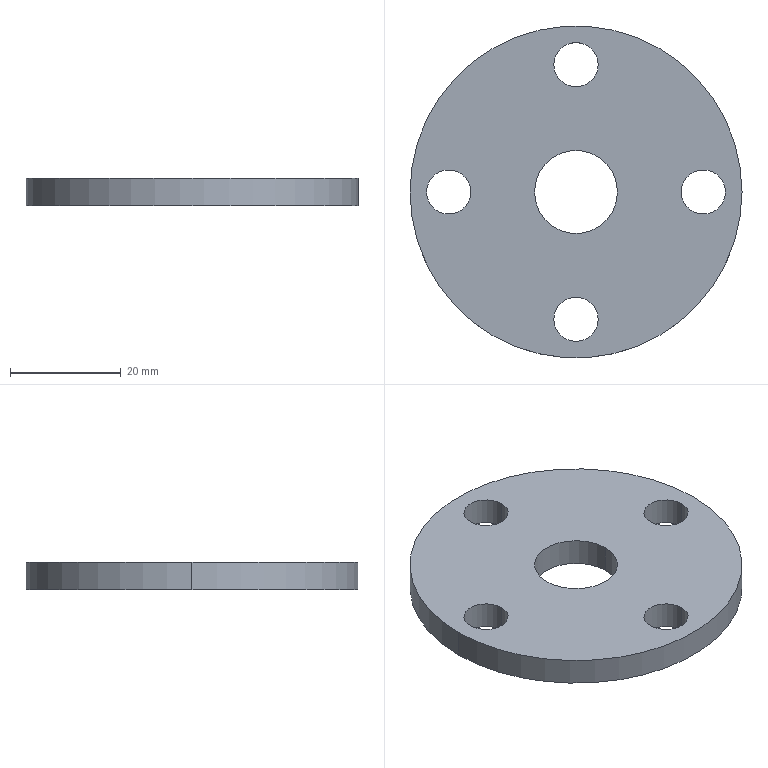Part | NX | features BREP 1 | 1 solid | 14 faces | box 60 x 60 x 5 mm | volume 12248 mm3 | cylinder 12 | plane 2 | commonest cylinder face diameters 8 x8 15 x2 60 x2
STEP:
#1=CARTESIAN_POINT('',(-27.,0.,5.));
#2=VERTEX_POINT('',#1);
#3=CARTESIAN_POINT('',(-19.,0.,5.));
#4=VERTEX_POINT('',#3);
#5=CARTESIAN_POINT('',(-23.,0.,5.));
#6=DIRECTION('',(0.,0.,1.));
#7=DIRECTION('',(1.,0.,0.));
#8=AXIS2_PLACEMENT_3D('',#5,#6,#7);
#9=CIRCLE('',#8,4.);
#10=EDGE_CURVE('',#2,#4,#9,.T.);
#11=ORIENTED_EDGE('',*,*,#10,.T.);
#12=CARTESIAN_POINT('',(-19.,0.,0.));
#13=VERTEX_POINT('',#12);
#14=CARTESIAN_POINT('',(-19.,0.,5.));
#15=DIRECTION('',(0.,0.,-1.));
#16=VECTOR('',#15,1000.);
#17=LINE('',#14,#16);
#18=EDGE_CURVE('',#13,#4,#17,.F.);
#19=ORIENTED_EDGE('',*,*,#18,.F.);
#20=CARTESIAN_POINT('',(-27.,0.,0.));
#21=VERTEX_POINT('',#20);
#22=CARTESIAN_POINT('',(-23.,0.,0.));
#23=DIRECTION('',(0.,0.,1.));
#24=DIRECTION('',(1.,0.,0.));
#25=AXIS2_PLACEMENT_3D('',#22,#23,#24);
#26=CIRCLE('',#25,4.);
#27=EDGE_CURVE('',#21,#13,#26,.T.);
#28=ORIENTED_EDGE('',*,*,#27,.F.);
#29=CARTESIAN_POINT('',(-27.,0.,5.));
#30=DIRECTION('',(0.,0.,-1.));
#31=VECTOR('',#30,1000.);
#32=LINE('',#29,#31);
#33=EDGE_CURVE('',#21,#2,#32,.F.);
#34=ORIENTED_EDGE('',*,*,#33,.T.);
#35=EDGE_LOOP('',(#11,#19,#28,#34));
#36=FACE_BOUND('',#35,.T.);
#37=CARTESIAN_POINT('',(-23.,0.,5.));
#38=DIRECTION('',(0.,0.,-1.));
#39=DIRECTION('',(1.,0.,0.));
#40=AXIS2_PLACEMENT_3D('',#37,#38,#39);
#41=CYLINDRICAL_SURFACE('',#40,4.);
#42=ADVANCED_FACE('',(#36),#41,.F.);
#43=CARTESIAN_POINT('',(-4.,-23.,5.));
#44=VERTEX_POINT('',#43);
#45=CARTESIAN_POINT('',(4.,-23.,5.));
#46=VERTEX_POINT('',#45);
#47=CARTESIAN_POINT('',(0.,-23.,5.));
#48=DIRECTION('',(0.,0.,1.));
#49=DIRECTION('',(1.,0.,0.));
#50=AXIS2_PLACEMENT_3D('',#47,#48,#49);
#51=CIRCLE('',#50,4.);
#52=EDGE_CURVE('',#44,#46,#51,.T.);
#53=ORIENTED_EDGE('',*,*,#52,.T.);
#54=CARTESIAN_POINT('',(4.,-23.,0.));
#55=VERTEX_POINT('',#54);
#56=CARTESIAN_POINT('',(4.,-23.,5.));
#57=DIRECTION('',(0.,0.,-1.));
#58=VECTOR('',#57,1000.);
#59=LINE('',#56,#58);
#60=EDGE_CURVE('',#55,#46,#59,.F.);
#61=ORIENTED_EDGE('',*,*,#60,.F.);
#62=CARTESIAN_POINT('',(-4.,-23.,0.));
#63=VERTEX_POINT('',#62);
#64=CARTESIAN_POINT('',(0.,-23.,0.));
#65=DIRECTION('',(0.,0.,1.));
#66=DIRECTION('',(1.,0.,0.));
#67=AXIS2_PLACEMENT_3D('',#64,#65,#66);
#68=CIRCLE('',#67,4.);
#69=EDGE_CURVE('',#63,#55,#68,.T.);
#70=ORIENTED_EDGE('',*,*,#69,.F.);
#71=CARTESIAN_POINT('',(-4.,-23.,5.));
#72=DIRECTION('',(0.,0.,-1.));
#73=VECTOR('',#72,1000.);
#74=LINE('',#71,#73);
#75=EDGE_CURVE('',#63,#44,#74,.F.);
#76=ORIENTED_EDGE('',*,*,#75,.T.);
#77=EDGE_LOOP('',(#53,#61,#70,#76));
#78=FACE_BOUND('',#77,.T.);
#79=CARTESIAN_POINT('',(0.,-23.,5.));
#80=DIRECTION('',(0.,0.,-1.));
#81=DIRECTION('',(1.,0.,0.));
#82=AXIS2_PLACEMENT_3D('',#79,#80,#81);
#83=CYLINDRICAL_SURFACE('',#82,4.);
#84=ADVANCED_FACE('',(#78),#83,.F.);
#85=CARTESIAN_POINT('',(19.,0.,5.));
#86=VERTEX_POINT('',#85);
#87=CARTESIAN_POINT('',(27.,0.,5.));
#88=VERTEX_POINT('',#87);
#89=CARTESIAN_POINT('',(23.,0.,5.));
#90=DIRECTION('',(0.,0.,1.));
#91=DIRECTION('',(1.,0.,0.));
#92=AXIS2_PLACEMENT_3D('',#89,#90,#91);
#93=CIRCLE('',#92,4.);
#94=EDGE_CURVE('',#86,#88,#93,.T.);
#95=ORIENTED_EDGE('',*,*,#94,.T.);
#96=CARTESIAN_POINT('',(27.,0.,0.));
#97=VERTEX_POINT('',#96);
#98=CARTESIAN_POINT('',(27.,0.,5.));
#99=DIRECTION('',(0.,0.,-1.));
#100=VECTOR('',#99,1000.);
#101=LINE('',#98,#100);
#102=EDGE_CURVE('',#97,#88,#101,.F.);
#103=ORIENTED_EDGE('',*,*,#102,.F.);
#104=CARTESIAN_POINT('',(19.,0.,0.));
#105=VERTEX_POINT('',#104);
#106=CARTESIAN_POINT('',(23.,0.,0.));
#107=DIRECTION('',(0.,0.,1.));
#108=DIRECTION('',(1.,0.,0.));
#109=AXIS2_PLACEMENT_3D('',#106,#107,#108);
#110=CIRCLE('',#109,4.);
#111=EDGE_CURVE('',#105,#97,#110,.T.);
#112=ORIENTED_EDGE('',*,*,#111,.F.);
#113=CARTESIAN_POINT('',(19.,0.,5.));
#114=DIRECTION('',(0.,0.,-1.));
#115=VECTOR('',#114,1000.);
#116=LINE('',#113,#115);
#117=EDGE_CURVE('',#105,#86,#116,.F.);
#118=ORIENTED_EDGE('',*,*,#117,.T.);
#119=EDGE_LOOP('',(#95,#103,#112,#118));
#120=FACE_BOUND('',#119,.T.);
#121=CARTESIAN_POINT('',(23.,0.,5.));
#122=DIRECTION('',(0.,0.,-1.));
#123=DIRECTION('',(1.,0.,0.));
#124=AXIS2_PLACEMENT_3D('',#121,#122,#123);
#125=CYLINDRICAL_SURFACE('',#124,4.);
#126=ADVANCED_FACE('',(#120),#125,.F.);
#127=CARTESIAN_POINT('',(-7.5,0.,5.));
#128=VERTEX_POINT('',#127);
#129=CARTESIAN_POINT('',(7.5,0.,5.));
#130=VERTEX_POINT('',#129);
#131=CARTESIAN_POINT('',(0.,0.,5.));
#132=DIRECTION('',(0.,0.,1.));
#133=DIRECTION('',(1.,0.,0.));
#134=AXIS2_PLACEMENT_3D('',#131,#132,#133);
#135=CIRCLE('',#134,7.5);
#136=EDGE_CURVE('',#128,#130,#135,.T.);
#137=ORIENTED_EDGE('',*,*,#136,.T.);
#138=CARTESIAN_POINT('',(7.5,0.,0.));
#139=VERTEX_POINT('',#138);
#140=CARTESIAN_POINT('',(7.5,0.,5.));
#141=DIRECTION('',(0.,0.,-1.));
#142=VECTOR('',#141,1000.);
#143=LINE('',#140,#142);
#144=EDGE_CURVE('',#139,#130,#143,.F.);
#145=ORIENTED_EDGE('',*,*,#144,.F.);
#146=CARTESIAN_POINT('',(-7.5,0.,0.));
#147=VERTEX_POINT('',#146);
#148=CARTESIAN_POINT('',(0.,0.,0.));
#149=DIRECTION('',(0.,0.,1.));
#150=DIRECTION('',(1.,0.,0.));
#151=AXIS2_PLACEMENT_3D('',#148,#149,#150);
#152=CIRCLE('',#151,7.5);
#153=EDGE_CURVE('',#147,#139,#152,.T.);
#154=ORIENTED_EDGE('',*,*,#153,.F.);
#155=CARTESIAN_POINT('',(-7.5,0.,5.));
#156=DIRECTION('',(0.,0.,-1.));
#157=VECTOR('',#156,1000.);
#158=LINE('',#155,#157);
#159=EDGE_CURVE('',#147,#128,#158,.F.);
#160=ORIENTED_EDGE('',*,*,#159,.T.);
#161=EDGE_LOOP('',(#137,#145,#154,#160));
#162=FACE_BOUND('',#161,.T.);
#163=CARTESIAN_POINT('',(0.,0.,5.));
#164=DIRECTION('',(0.,0.,-1.));
#165=DIRECTION('',(1.,0.,0.));
#166=AXIS2_PLACEMENT_3D('',#163,#164,#165);
#167=CYLINDRICAL_SURFACE('',#166,7.5);
#168=ADVANCED_FACE('',(#162),#167,.F.);
#169=CARTESIAN_POINT('',(-4.,23.,5.));
#170=VERTEX_POINT('',#169);
#171=CARTESIAN_POINT('',(4.,23.,5.));
#172=VERTEX_POINT('',#171);
#173=CARTESIAN_POINT('',(0.,23.,5.));
#174=DIRECTION('',(0.,0.,1.));
#175=DIRECTION('',(1.,0.,0.));
#176=AXIS2_PLACEMENT_3D('',#173,#174,#175);
#177=CIRCLE('',#176,4.);
#178=EDGE_CURVE('',#170,#172,#177,.T.);
#179=ORIENTED_EDGE('',*,*,#178,.T.);
#180=CARTESIAN_POINT('',(4.,23.,0.));
#181=VERTEX_POINT('',#180);
#182=CARTESIAN_POINT('',(4.,23.,5.));
#183=DIRECTION('',(0.,0.,-1.));
#184=VECTOR('',#183,1000.);
#185=LINE('',#182,#184);
#186=EDGE_CURVE('',#181,#172,#185,.F.);
#187=ORIENTED_EDGE('',*,*,#186,.F.);
#188=CARTESIAN_POINT('',(-4.,23.,0.));
#189=VERTEX_POINT('',#188);
#190=CARTESIAN_POINT('',(0.,23.,0.));
#191=DIRECTION('',(0.,0.,1.));
#192=DIRECTION('',(1.,0.,0.));
#193=AXIS2_PLACEMENT_3D('',#190,#191,#192);
#194=CIRCLE('',#193,4.);
#195=EDGE_CURVE('',#189,#181,#194,.T.);
#196=ORIENTED_EDGE('',*,*,#195,.F.);
#197=CARTESIAN_POINT('',(-4.,23.,5.));
#198=DIRECTION('',(0.,0.,-1.));
#199=VECTOR('',#198,1000.);
#200=LINE('',#197,#199);
#201=EDGE_CURVE('',#189,#170,#200,.F.);
#202=ORIENTED_EDGE('',*,*,#201,.T.);
#203=EDGE_LOOP('',(#179,#187,#196,#202));
#204=FACE_BOUND('',#203,.T.);
#205=CARTESIAN_POINT('',(0.,23.,5.));
#206=DIRECTION('',(0.,0.,-1.));
#207=DIRECTION('',(1.,0.,0.));
#208=AXIS2_PLACEMENT_3D('',#205,#206,#207);
#209=CYLINDRICAL_SURFACE('',#208,4.);
#210=ADVANCED_FACE('',(#204),#209,.F.);
#211=CARTESIAN_POINT('',(30.,0.,5.));
#212=VERTEX_POINT('',#211);
#213=CARTESIAN_POINT('',(-30.,0.,5.));
#214=VERTEX_POINT('',#213);
#215=CARTESIAN_POINT('',(0.,0.,5.));
#216=DIRECTION('',(0.,0.,1.));
#217=DIRECTION('',(1.,0.,0.));
#218=AXIS2_PLACEMENT_3D('',#215,#216,#217);
#219=CIRCLE('',#218,30.);
#220=EDGE_CURVE('',#212,#214,#219,.T.);
#221=ORIENTED_EDGE('',*,*,#220,.F.);
#222=CARTESIAN_POINT('',(30.,0.,0.));
#223=VERTEX_POINT('',#222);
#224=CARTESIAN_POINT('',(30.,0.,5.));
#225=DIRECTION('',(0.,0.,-1.));
#226=VECTOR('',#225,1000.);
#227=LINE('',#224,#226);
#228=EDGE_CURVE('',#223,#212,#227,.F.);
#229=ORIENTED_EDGE('',*,*,#228,.F.);
#230=CARTESIAN_POINT('',(-30.,0.,0.));
#231=VERTEX_POINT('',#230);
#232=CARTESIAN_POINT('',(0.,0.,0.));
#233=DIRECTION('',(0.,0.,1.));
#234=DIRECTION('',(1.,0.,0.));
#235=AXIS2_PLACEMENT_3D('',#232,#233,#234);
#236=CIRCLE('',#235,30.);
#237=EDGE_CURVE('',#223,#231,#236,.T.);
#238=ORIENTED_EDGE('',*,*,#237,.T.);
#239=CARTESIAN_POINT('',(-30.,0.,5.));
#240=DIRECTION('',(0.,0.,-1.));
#241=VECTOR('',#240,1000.);
#242=LINE('',#239,#241);
#243=EDGE_CURVE('',#231,#214,#242,.F.);
#244=ORIENTED_EDGE('',*,*,#243,.T.);
#245=EDGE_LOOP('',(#221,#229,#238,#244));
#246=FACE_BOUND('',#245,.T.);
#247=CARTESIAN_POINT('',(0.,0.,5.));
#248=DIRECTION('',(0.,0.,-1.));
#249=DIRECTION('',(1.,0.,0.));
#250=AXIS2_PLACEMENT_3D('',#247,#248,#249);
#251=CYLINDRICAL_SURFACE('',#250,30.);
#252=ADVANCED_FACE('',(#246),#251,.T.);
#253=CARTESIAN_POINT('',(0.,0.,5.));
#254=DIRECTION('',(0.,0.,1.));
#255=DIRECTION('',(1.,0.,0.));
#256=AXIS2_PLACEMENT_3D('',#253,#254,#255);
#257=CIRCLE('',#256,30.);
#258=EDGE_CURVE('',#214,#212,#257,.T.);
#259=ORIENTED_EDGE('',*,*,#258,.T.);
#260=ORIENTED_EDGE('',*,*,#220,.T.);
#261=EDGE_LOOP('',(#259,#260));
#262=FACE_BOUND('',#261,.T.);
#263=ORIENTED_EDGE('',*,*,#52,.F.);
#264=CARTESIAN_POINT('',(0.,-23.,5.));
#265=DIRECTION('',(0.,0.,1.));
#266=DIRECTION('',(1.,0.,0.));
#267=AXIS2_PLACEMENT_3D('',#264,#265,#266);
#268=CIRCLE('',#267,4.);
#269=EDGE_CURVE('',#46,#44,#268,.T.);
#270=ORIENTED_EDGE('',*,*,#269,.F.);
#271=EDGE_LOOP('',(#263,#270));
#272=FACE_BOUND('',#271,.T.);
#273=ORIENTED_EDGE('',*,*,#136,.F.);
#274=CARTESIAN_POINT('',(0.,0.,5.));
#275=DIRECTION('',(0.,0.,1.));
#276=DIRECTION('',(1.,0.,0.));
#277=AXIS2_PLACEMENT_3D('',#274,#275,#276);
#278=CIRCLE('',#277,7.5);
#279=EDGE_CURVE('',#130,#128,#278,.T.);
#280=ORIENTED_EDGE('',*,*,#279,.F.);
#281=EDGE_LOOP('',(#273,#280));
#282=FACE_BOUND('',#281,.T.);
#283=ORIENTED_EDGE('',*,*,#178,.F.);
#284=CARTESIAN_POINT('',(0.,23.,5.));
#285=DIRECTION('',(0.,0.,1.));
#286=DIRECTION('',(1.,0.,0.));
#287=AXIS2_PLACEMENT_3D('',#284,#285,#286);
#288=CIRCLE('',#287,4.);
#289=EDGE_CURVE('',#172,#170,#288,.T.);
#290=ORIENTED_EDGE('',*,*,#289,.F.);
#291=EDGE_LOOP('',(#283,#290));
#292=FACE_BOUND('',#291,.T.);
#293=ORIENTED_EDGE('',*,*,#94,.F.);
#294=CARTESIAN_POINT('',(23.,0.,5.));
#295=DIRECTION('',(0.,0.,1.));
#296=DIRECTION('',(1.,0.,0.));
#297=AXIS2_PLACEMENT_3D('',#294,#295,#296);
#298=CIRCLE('',#297,4.);
#299=EDGE_CURVE('',#88,#86,#298,.T.);
#300=ORIENTED_EDGE('',*,*,#299,.F.);
#301=EDGE_LOOP('',(#293,#300));
#302=FACE_BOUND('',#301,.T.);
#303=ORIENTED_EDGE('',*,*,#10,.F.);
#304=CARTESIAN_POINT('',(-23.,0.,5.));
#305=DIRECTION('',(0.,0.,1.));
#306=DIRECTION('',(1.,0.,0.));
#307=AXIS2_PLACEMENT_3D('',#304,#305,#306);
#308=CIRCLE('',#307,4.);
#309=EDGE_CURVE('',#4,#2,#308,.T.);
#310=ORIENTED_EDGE('',*,*,#309,.F.);
#311=EDGE_LOOP('',(#303,#310));
#312=FACE_BOUND('',#311,.T.);
#313=CARTESIAN_POINT('',(0.,0.,5.));
#314=DIRECTION('',(0.,0.,1.));
#315=DIRECTION('',(0.,1.,0.));
#316=AXIS2_PLACEMENT_3D('',#313,#314,#315);
#317=PLANE('',#316);
#318=ADVANCED_FACE('',(#262,#272,#282,#292,#302,#312),#317,.T.);
#319=CARTESIAN_POINT('',(0.,0.,0.));
#320=DIRECTION('',(0.,0.,1.));
#321=DIRECTION('',(1.,0.,0.));
#322=AXIS2_PLACEMENT_3D('',#319,#320,#321);
#323=CIRCLE('',#322,30.);
#324=EDGE_CURVE('',#231,#223,#323,.T.);
#325=ORIENTED_EDGE('',*,*,#324,.F.);
#326=ORIENTED_EDGE('',*,*,#237,.F.);
#327=EDGE_LOOP('',(#325,#326));
#328=FACE_BOUND('',#327,.T.);
#329=ORIENTED_EDGE('',*,*,#69,.T.);
#330=CARTESIAN_POINT('',(0.,-23.,0.));
#331=DIRECTION('',(0.,0.,1.));
#332=DIRECTION('',(1.,0.,0.));
#333=AXIS2_PLACEMENT_3D('',#330,#331,#332);
#334=CIRCLE('',#333,4.);
#335=EDGE_CURVE('',#55,#63,#334,.T.);
#336=ORIENTED_EDGE('',*,*,#335,.T.);
#337=EDGE_LOOP('',(#329,#336));
#338=FACE_BOUND('',#337,.T.);
#339=ORIENTED_EDGE('',*,*,#153,.T.);
#340=CARTESIAN_POINT('',(0.,0.,0.));
#341=DIRECTION('',(0.,0.,1.));
#342=DIRECTION('',(1.,0.,0.));
#343=AXIS2_PLACEMENT_3D('',#340,#341,#342);
#344=CIRCLE('',#343,7.5);
#345=EDGE_CURVE('',#139,#147,#344,.T.);
#346=ORIENTED_EDGE('',*,*,#345,.T.);
#347=EDGE_LOOP('',(#339,#346));
#348=FACE_BOUND('',#347,.T.);
#349=ORIENTED_EDGE('',*,*,#195,.T.);
#350=CARTESIAN_POINT('',(0.,23.,0.));
#351=DIRECTION('',(0.,0.,1.));
#352=DIRECTION('',(1.,0.,0.));
#353=AXIS2_PLACEMENT_3D('',#350,#351,#352);
#354=CIRCLE('',#353,4.);
#355=EDGE_CURVE('',#181,#189,#354,.T.);
#356=ORIENTED_EDGE('',*,*,#355,.T.);
#357=EDGE_LOOP('',(#349,#356));
#358=FACE_BOUND('',#357,.T.);
#359=ORIENTED_EDGE('',*,*,#111,.T.);
#360=CARTESIAN_POINT('',(23.,0.,0.));
#361=DIRECTION('',(0.,0.,1.));
#362=DIRECTION('',(1.,0.,0.));
#363=AXIS2_PLACEMENT_3D('',#360,#361,#362);
#364=CIRCLE('',#363,4.);
#365=EDGE_CURVE('',#97,#105,#364,.T.);
#366=ORIENTED_EDGE('',*,*,#365,.T.);
#367=EDGE_LOOP('',(#359,#366));
#368=FACE_BOUND('',#367,.T.);
#369=ORIENTED_EDGE('',*,*,#27,.T.);
#370=CARTESIAN_POINT('',(-23.,0.,0.));
#371=DIRECTION('',(0.,0.,1.));
#372=DIRECTION('',(1.,0.,0.));
#373=AXIS2_PLACEMENT_3D('',#370,#371,#372);
#374=CIRCLE('',#373,4.);
#375=EDGE_CURVE('',#13,#21,#374,.T.);
#376=ORIENTED_EDGE('',*,*,#375,.T.);
#377=EDGE_LOOP('',(#369,#376));
#378=FACE_BOUND('',#377,.T.);
#379=CARTESIAN_POINT('',(0.,0.,0.));
#380=DIRECTION('',(0.,0.,1.));
#381=DIRECTION('',(0.,1.,0.));
#382=AXIS2_PLACEMENT_3D('',#379,#380,#381);
#383=PLANE('',#382);
#384=ADVANCED_FACE('',(#328,#338,#348,#358,#368,#378),#383,.F.);
#385=ORIENTED_EDGE('',*,*,#228,.T.);
#386=ORIENTED_EDGE('',*,*,#258,.F.);
#387=ORIENTED_EDGE('',*,*,#243,.F.);
#388=ORIENTED_EDGE('',*,*,#324,.T.);
#389=EDGE_LOOP('',(#385,#386,#387,#388));
#390=FACE_BOUND('',#389,.T.);
#391=CARTESIAN_POINT('',(0.,0.,5.));
#392=DIRECTION('',(0.,0.,-1.));
#393=DIRECTION('',(1.,0.,0.));
#394=AXIS2_PLACEMENT_3D('',#391,#392,#393);
#395=CYLINDRICAL_SURFACE('',#394,30.);
#396=ADVANCED_FACE('',(#390),#395,.T.);
#397=ORIENTED_EDGE('',*,*,#186,.T.);
#398=ORIENTED_EDGE('',*,*,#289,.T.);
#399=ORIENTED_EDGE('',*,*,#201,.F.);
#400=ORIENTED_EDGE('',*,*,#355,.F.);
#401=EDGE_LOOP('',(#397,#398,#399,#400));
#402=FACE_BOUND('',#401,.T.);
#403=CARTESIAN_POINT('',(0.,23.,5.));
#404=DIRECTION('',(0.,0.,-1.));
#405=DIRECTION('',(1.,0.,0.));
#406=AXIS2_PLACEMENT_3D('',#403,#404,#405);
#407=CYLINDRICAL_SURFACE('',#406,4.);
#408=ADVANCED_FACE('',(#402),#407,.F.);
#409=ORIENTED_EDGE('',*,*,#144,.T.);
#410=ORIENTED_EDGE('',*,*,#279,.T.);
#411=ORIENTED_EDGE('',*,*,#159,.F.);
#412=ORIENTED_EDGE('',*,*,#345,.F.);
#413=EDGE_LOOP('',(#409,#410,#411,#412));
#414=FACE_BOUND('',#413,.T.);
#415=CARTESIAN_POINT('',(0.,0.,5.));
#416=DIRECTION('',(0.,0.,-1.));
#417=DIRECTION('',(1.,0.,0.));
#418=AXIS2_PLACEMENT_3D('',#415,#416,#417);
#419=CYLINDRICAL_SURFACE('',#418,7.5);
#420=ADVANCED_FACE('',(#414),#419,.F.);
#421=ORIENTED_EDGE('',*,*,#102,.T.);
#422=ORIENTED_EDGE('',*,*,#299,.T.);
#423=ORIENTED_EDGE('',*,*,#117,.F.);
#424=ORIENTED_EDGE('',*,*,#365,.F.);
#425=EDGE_LOOP('',(#421,#422,#423,#424));
#426=FACE_BOUND('',#425,.T.);
#427=CARTESIAN_POINT('',(23.,0.,5.));
#428=DIRECTION('',(0.,0.,-1.));
#429=DIRECTION('',(1.,0.,0.));
#430=AXIS2_PLACEMENT_3D('',#427,#428,#429);
#431=CYLINDRICAL_SURFACE('',#430,4.);
#432=ADVANCED_FACE('',(#426),#431,.F.);
#433=ORIENTED_EDGE('',*,*,#60,.T.);
#434=ORIENTED_EDGE('',*,*,#269,.T.);
#435=ORIENTED_EDGE('',*,*,#75,.F.);
#436=ORIENTED_EDGE('',*,*,#335,.F.);
#437=EDGE_LOOP('',(#433,#434,#435,#436));
#438=FACE_BOUND('',#437,.T.);
#439=CARTESIAN_POINT('',(0.,-23.,5.));
#440=DIRECTION('',(0.,0.,-1.));
#441=DIRECTION('',(1.,0.,0.));
#442=AXIS2_PLACEMENT_3D('',#439,#440,#441);
#443=CYLINDRICAL_SURFACE('',#442,4.);
#444=ADVANCED_FACE('',(#438),#443,.F.);
#445=ORIENTED_EDGE('',*,*,#18,.T.);
#446=ORIENTED_EDGE('',*,*,#309,.T.);
#447=ORIENTED_EDGE('',*,*,#33,.F.);
#448=ORIENTED_EDGE('',*,*,#375,.F.);
#449=EDGE_LOOP('',(#445,#446,#447,#448));
#450=FACE_BOUND('',#449,.T.);
#451=CARTESIAN_POINT('',(-23.,0.,5.));
#452=DIRECTION('',(0.,0.,-1.));
#453=DIRECTION('',(1.,0.,0.));
#454=AXIS2_PLACEMENT_3D('',#451,#452,#453);
#455=CYLINDRICAL_SURFACE('',#454,4.);
#456=ADVANCED_FACE('',(#450),#455,.F.);
#457=CLOSED_SHELL('',(#42,#84,#126,#168,#210,#252,#318,#384,#396,#408,#420,#432,#444,#456));
#458=MANIFOLD_SOLID_BREP('',#457);
#459=(LENGTH_UNIT()NAMED_UNIT(*)SI_UNIT(.MILLI.,.METRE.));
#460=UNCERTAINTY_MEASURE_WITH_UNIT(LENGTH_MEASURE(0.00001),#459,'','');
#461=(NAMED_UNIT(*)PLANE_ANGLE_UNIT()SI_UNIT($,.RADIAN.));
#462=(NAMED_UNIT(*)SI_UNIT($,.STERADIAN.)SOLID_ANGLE_UNIT());
#463=(GEOMETRIC_REPRESENTATION_CONTEXT(3)GLOBAL_UNCERTAINTY_ASSIGNED_CONTEXT((#460))GLOBAL_UNIT_ASSIGNED_CONTEXT((#459,#461,#462))REPRESENTATION_CONTEXT('',''));
#464=ADVANCED_BREP_SHAPE_REPRESENTATION('',(#458),#463);